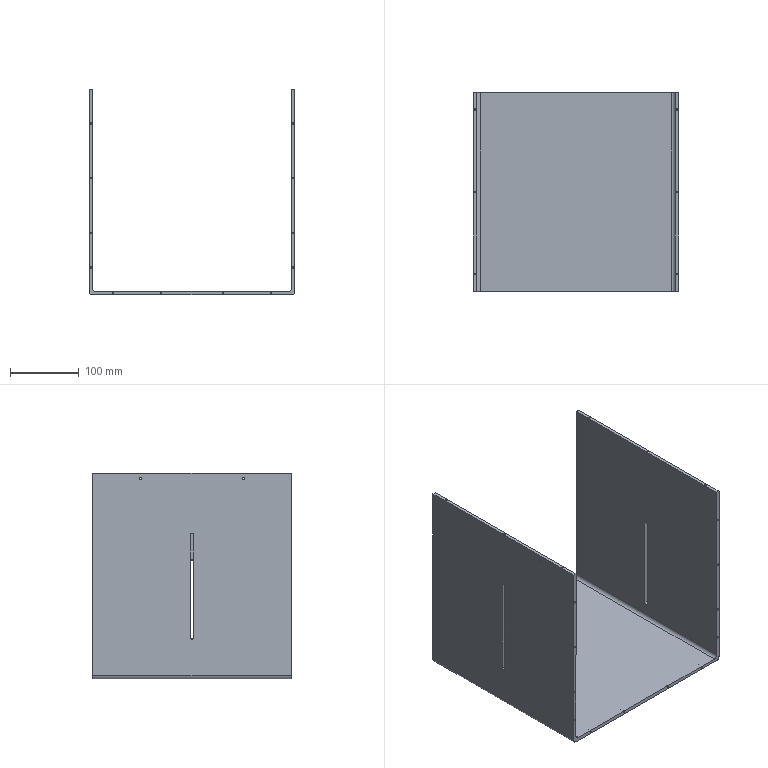Part | SolidWorks | features HoleWzd 3, ICE 2, Extrusion 1 | 1 solid | 108 faces | box 300 x 290 x 300 mm | volume 1282164 mm3 | cylinder 54 | cone 40 | plane 14 | commonest cylinder face diameters 2.05 x36 3.3 x8 10 x4 4.2 x3 6.2 x3